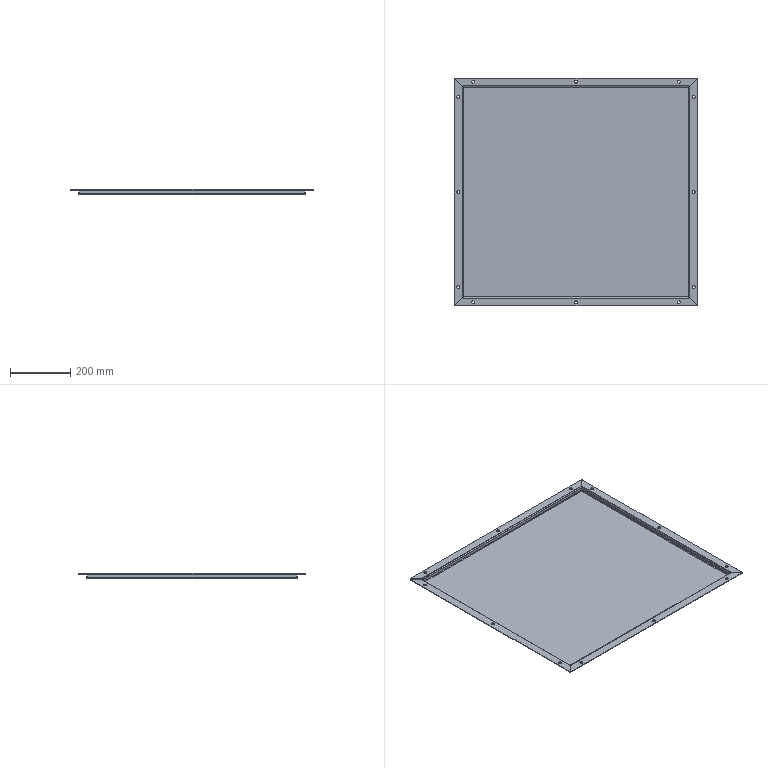Part | STEP file | 750078273 | 1 solid | 102 faces | box 811 x 758 x 17 mm | volume 1299071 mm3 | plane 54 | cylinder 48 | commonest cylinder face diameters 10 x32 4 x8 8 x8